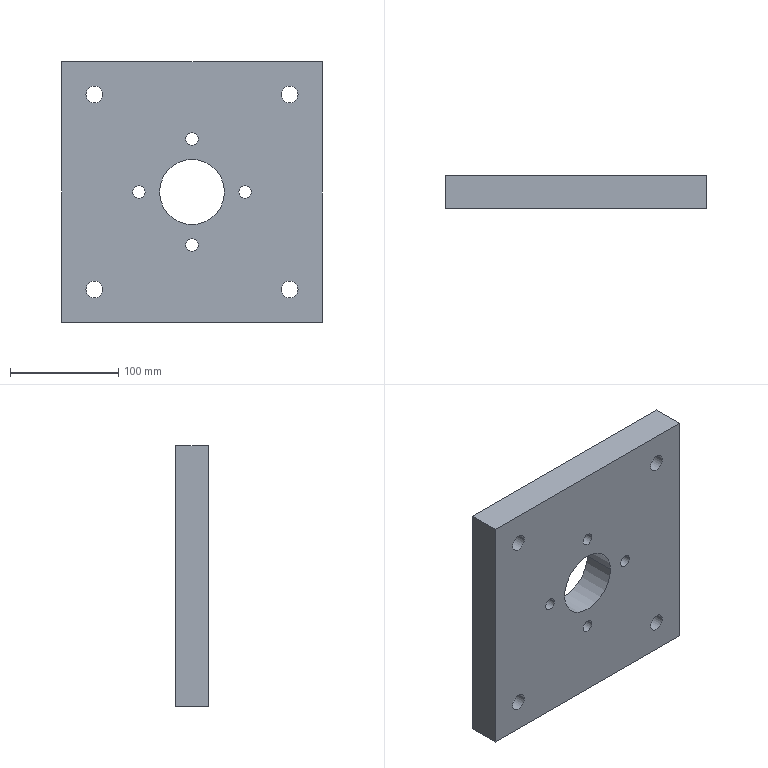Part | STEP file | Scale factor 1[5] | 1 solid | 32 faces | box 240 x 30 x 240 mm | volume 1602106 mm3 | cylinder 22 | plane 6 | cone 4 | commonest cylinder face diameters 11.4 x8 15.6 x8 10.2 x4 60 x2
STEP:
#1=CARTESIAN_POINT('',(-808.738,-386.273,3156.564));
#2=VERTEX_POINT('',#1);
#3=CARTESIAN_POINT('',(-808.738,-381.173,3153.5));
#4=VERTEX_POINT('',#3);
#5=CARTESIAN_POINT('',(-808.738,-381.173,3153.5));
#6=DIRECTION('',(0.,0.8572,-0.515));
#7=VECTOR('',#6,1000.);
#8=LINE('',#5,#7);
#9=EDGE_CURVE('',#2,#4,#8,.T.);
#10=ORIENTED_EDGE('',*,*,#9,.F.);
#11=CARTESIAN_POINT('',(-808.738,-391.373,3153.5));
#12=VERTEX_POINT('',#11);
#13=CARTESIAN_POINT('',(-808.738,-391.373,3153.5));
#14=DIRECTION('',(0.,-0.8572,-0.515));
#15=VECTOR('',#14,1000.);
#16=LINE('',#13,#15);
#17=EDGE_CURVE('',#2,#12,#16,.T.);
#18=ORIENTED_EDGE('',*,*,#17,.T.);
#19=CARTESIAN_POINT('',(-808.738,-386.273,3153.5));
#20=DIRECTION('',(0.,0.,-1.));
#21=DIRECTION('',(0.,1.,0.));
#22=AXIS2_PLACEMENT_3D('',#19,#20,#21);
#23=CIRCLE('',#22,5.1);
#24=EDGE_CURVE('',#12,#4,#23,.T.);
#25=ORIENTED_EDGE('',*,*,#24,.T.);
#26=EDGE_LOOP('',(#10,#18,#25));
#27=FACE_OUTER_BOUND('',#26,.T.);
#28=CARTESIAN_POINT('',(-808.738,-386.273,3153.5));
#29=DIRECTION('',(0.,0.,-1.));
#30=DIRECTION('',(0.,-1.,0.));
#31=AXIS2_PLACEMENT_3D('',#28,#29,#30);
#32=CONICAL_SURFACE('',#31,5.1,1.03);
#33=ADVANCED_FACE('',(#27),#32,.F.);
#34=ORIENTED_EDGE('',*,*,#24,.F.);
#35=CARTESIAN_POINT('',(-808.738,-391.373,3118.5));
#36=VERTEX_POINT('',#35);
#37=CARTESIAN_POINT('',(-808.738,-391.373,3083.5));
#38=DIRECTION('',(0.,0.,-1.));
#39=VECTOR('',#38,1000.);
#40=LINE('',#37,#39);
#41=EDGE_CURVE('',#12,#36,#40,.T.);
#42=ORIENTED_EDGE('',*,*,#41,.T.);
#43=CARTESIAN_POINT('',(-808.738,-381.173,3118.5));
#44=VERTEX_POINT('',#43);
#45=CARTESIAN_POINT('',(-808.738,-386.273,3118.5));
#46=DIRECTION('',(-0.000000001,0.,1.));
#47=DIRECTION('',(0.,-1.,0.));
#48=AXIS2_PLACEMENT_3D('',#45,#46,#47);
#49=CIRCLE('',#48,5.1);
#50=EDGE_CURVE('',#44,#36,#49,.T.);
#51=ORIENTED_EDGE('',*,*,#50,.F.);
#52=CARTESIAN_POINT('',(-808.738,-381.173,3083.5));
#53=DIRECTION('',(0.,0.,-1.));
#54=VECTOR('',#53,1000.);
#55=LINE('',#52,#54);
#56=EDGE_CURVE('',#4,#44,#55,.T.);
#57=ORIENTED_EDGE('',*,*,#56,.F.);
#58=EDGE_LOOP('',(#34,#42,#51,#57));
#59=FACE_OUTER_BOUND('',#58,.T.);
#60=CARTESIAN_POINT('',(-808.738,-386.273,3083.5));
#61=DIRECTION('',(0.,0.,-1.));
#62=DIRECTION('',(0.,-1.,0.));
#63=AXIS2_PLACEMENT_3D('',#60,#61,#62);
#64=CYLINDRICAL_SURFACE('',#63,5.1);
#65=ADVANCED_FACE('',(#59),#64,.F.);
#66=CARTESIAN_POINT('',(-688.738,-386.273,3156.564));
#67=VERTEX_POINT('',#66);
#68=CARTESIAN_POINT('',(-688.738,-381.173,3153.5));
#69=VERTEX_POINT('',#68);
#70=CARTESIAN_POINT('',(-688.738,-381.173,3153.5));
#71=DIRECTION('',(0.,0.8572,-0.515));
#72=VECTOR('',#71,1000.);
#73=LINE('',#70,#72);
#74=EDGE_CURVE('',#67,#69,#73,.T.);
#75=ORIENTED_EDGE('',*,*,#74,.F.);
#76=CARTESIAN_POINT('',(-688.738,-391.373,3153.5));
#77=VERTEX_POINT('',#76);
#78=CARTESIAN_POINT('',(-688.738,-391.373,3153.5));
#79=DIRECTION('',(0.,-0.8572,-0.515));
#80=VECTOR('',#79,1000.);
#81=LINE('',#78,#80);
#82=EDGE_CURVE('',#67,#77,#81,.T.);
#83=ORIENTED_EDGE('',*,*,#82,.T.);
#84=CARTESIAN_POINT('',(-688.738,-386.273,3153.5));
#85=DIRECTION('',(0.,0.,-1.));
#86=DIRECTION('',(0.,1.,0.));
#87=AXIS2_PLACEMENT_3D('',#84,#85,#86);
#88=CIRCLE('',#87,5.1);
#89=EDGE_CURVE('',#77,#69,#88,.T.);
#90=ORIENTED_EDGE('',*,*,#89,.T.);
#91=EDGE_LOOP('',(#75,#83,#90));
#92=FACE_OUTER_BOUND('',#91,.T.);
#93=CARTESIAN_POINT('',(-688.738,-386.273,3153.5));
#94=DIRECTION('',(0.,0.,-1.));
#95=DIRECTION('',(0.,-1.,0.));
#96=AXIS2_PLACEMENT_3D('',#93,#94,#95);
#97=CONICAL_SURFACE('',#96,5.1,1.03);
#98=ADVANCED_FACE('',(#92),#97,.F.);
#99=ORIENTED_EDGE('',*,*,#89,.F.);
#100=CARTESIAN_POINT('',(-688.738,-391.373,3118.5));
#101=VERTEX_POINT('',#100);
#102=CARTESIAN_POINT('',(-688.738,-391.373,3083.5));
#103=DIRECTION('',(0.,0.,-1.));
#104=VECTOR('',#103,1000.);
#105=LINE('',#102,#104);
#106=EDGE_CURVE('',#77,#101,#105,.T.);
#107=ORIENTED_EDGE('',*,*,#106,.T.);
#108=CARTESIAN_POINT('',(-688.738,-381.173,3118.5));
#109=VERTEX_POINT('',#108);
#110=CARTESIAN_POINT('',(-688.738,-386.273,3118.5));
#111=DIRECTION('',(-0.000000001,0.,1.));
#112=DIRECTION('',(0.,-1.,0.));
#113=AXIS2_PLACEMENT_3D('',#110,#111,#112);
#114=CIRCLE('',#113,5.1);
#115=EDGE_CURVE('',#109,#101,#114,.T.);
#116=ORIENTED_EDGE('',*,*,#115,.F.);
#117=CARTESIAN_POINT('',(-688.738,-381.173,3083.5));
#118=DIRECTION('',(0.,0.,-1.));
#119=VECTOR('',#118,1000.);
#120=LINE('',#117,#119);
#121=EDGE_CURVE('',#69,#109,#120,.T.);
#122=ORIENTED_EDGE('',*,*,#121,.F.);
#123=EDGE_LOOP('',(#99,#107,#116,#122));
#124=FACE_OUTER_BOUND('',#123,.T.);
#125=CARTESIAN_POINT('',(-688.738,-386.273,3083.5));
#126=DIRECTION('',(0.,0.,-1.));
#127=DIRECTION('',(0.,-1.,0.));
#128=AXIS2_PLACEMENT_3D('',#125,#126,#127);
#129=CYLINDRICAL_SURFACE('',#128,5.1);
#130=ADVANCED_FACE('',(#124),#129,.F.);
#131=CARTESIAN_POINT('',(-778.738,-401.273,3238.5));
#132=VERTEX_POINT('',#131);
#133=CARTESIAN_POINT('',(-718.738,-401.273,3238.5));
#134=VERTEX_POINT('',#133);
#135=CARTESIAN_POINT('',(-748.738,-401.273,3238.5));
#136=DIRECTION('',(0.,1.,0.));
#137=DIRECTION('',(1.,0.,0.000000001));
#138=AXIS2_PLACEMENT_3D('',#135,#136,#137);
#139=CIRCLE('',#138,30.);
#140=EDGE_CURVE('',#132,#134,#139,.T.);
#141=ORIENTED_EDGE('',*,*,#140,.F.);
#142=CARTESIAN_POINT('',(-778.738,-371.273,3238.5));
#143=VERTEX_POINT('',#142);
#144=CARTESIAN_POINT('',(-778.738,-401.273,3238.5));
#145=DIRECTION('',(0.,1.,0.));
#146=VECTOR('',#145,1000.);
#147=LINE('',#144,#146);
#148=EDGE_CURVE('',#132,#143,#147,.T.);
#149=ORIENTED_EDGE('',*,*,#148,.T.);
#150=CARTESIAN_POINT('',(-718.738,-371.273,3238.5));
#151=VERTEX_POINT('',#150);
#152=CARTESIAN_POINT('',(-748.738,-371.273,3238.5));
#153=DIRECTION('',(0.,1.,0.));
#154=DIRECTION('',(1.,0.,0.000000001));
#155=AXIS2_PLACEMENT_3D('',#152,#153,#154);
#156=CIRCLE('',#155,30.);
#157=EDGE_CURVE('',#143,#151,#156,.T.);
#158=ORIENTED_EDGE('',*,*,#157,.T.);
#159=CARTESIAN_POINT('',(-718.738,-401.273,3238.5));
#160=DIRECTION('',(0.,1.,0.));
#161=VECTOR('',#160,1000.);
#162=LINE('',#159,#161);
#163=EDGE_CURVE('',#134,#151,#162,.T.);
#164=ORIENTED_EDGE('',*,*,#163,.F.);
#165=EDGE_LOOP('',(#141,#149,#158,#164));
#166=FACE_OUTER_BOUND('',#165,.T.);
#167=CARTESIAN_POINT('',(-748.738,-401.273,3238.5));
#168=DIRECTION('',(0.,1.,0.));
#169=DIRECTION('',(-1.,0.,-0.000000001));
#170=AXIS2_PLACEMENT_3D('',#167,#168,#169);
#171=CYLINDRICAL_SURFACE('',#170,30.);
#172=ADVANCED_FACE('',(#166),#171,.F.);
#173=CARTESIAN_POINT('',(-705.538,-401.273,3238.5));
#174=VERTEX_POINT('',#173);
#175=CARTESIAN_POINT('',(-694.138,-401.273,3238.5));
#176=VERTEX_POINT('',#175);
#177=CARTESIAN_POINT('',(-699.838,-401.273,3238.5));
#178=DIRECTION('',(0.,1.,0.));
#179=DIRECTION('',(1.,0.,0.000000001));
#180=AXIS2_PLACEMENT_3D('',#177,#178,#179);
#181=CIRCLE('',#180,5.7);
#182=EDGE_CURVE('',#174,#176,#181,.T.);
#183=ORIENTED_EDGE('',*,*,#182,.F.);
#184=CARTESIAN_POINT('',(-705.538,-371.273,3238.5));
#185=VERTEX_POINT('',#184);
#186=CARTESIAN_POINT('',(-705.538,-401.273,3238.5));
#187=DIRECTION('',(0.,1.,0.));
#188=VECTOR('',#187,1000.);
#189=LINE('',#186,#188);
#190=EDGE_CURVE('',#174,#185,#189,.T.);
#191=ORIENTED_EDGE('',*,*,#190,.T.);
#192=CARTESIAN_POINT('',(-694.138,-371.273,3238.5));
#193=VERTEX_POINT('',#192);
#194=CARTESIAN_POINT('',(-699.838,-371.273,3238.5));
#195=DIRECTION('',(0.,1.,0.));
#196=DIRECTION('',(1.,0.,0.000000001));
#197=AXIS2_PLACEMENT_3D('',#194,#195,#196);
#198=CIRCLE('',#197,5.7);
#199=EDGE_CURVE('',#185,#193,#198,.T.);
#200=ORIENTED_EDGE('',*,*,#199,.T.);
#201=CARTESIAN_POINT('',(-694.138,-401.273,3238.5));
#202=DIRECTION('',(0.,1.,0.));
#203=VECTOR('',#202,1000.);
#204=LINE('',#201,#203);
#205=EDGE_CURVE('',#176,#193,#204,.T.);
#206=ORIENTED_EDGE('',*,*,#205,.F.);
#207=EDGE_LOOP('',(#183,#191,#200,#206));
#208=FACE_OUTER_BOUND('',#207,.T.);
#209=CARTESIAN_POINT('',(-699.838,-401.273,3238.5));
#210=DIRECTION('',(0.,1.,0.));
#211=DIRECTION('',(-1.,0.,-0.000000001));
#212=AXIS2_PLACEMENT_3D('',#209,#210,#211);
#213=CYLINDRICAL_SURFACE('',#212,5.7);
#214=ADVANCED_FACE('',(#208),#213,.F.);
#215=CARTESIAN_POINT('',(-803.338,-401.273,3238.5));
#216=VERTEX_POINT('',#215);
#217=CARTESIAN_POINT('',(-791.938,-401.273,3238.5));
#218=VERTEX_POINT('',#217);
#219=CARTESIAN_POINT('',(-797.638,-401.273,3238.5));
#220=DIRECTION('',(0.,1.,0.));
#221=DIRECTION('',(1.,0.,0.000000001));
#222=AXIS2_PLACEMENT_3D('',#219,#220,#221);
#223=CIRCLE('',#222,5.7);
#224=EDGE_CURVE('',#216,#218,#223,.T.);
#225=ORIENTED_EDGE('',*,*,#224,.F.);
#226=CARTESIAN_POINT('',(-803.338,-371.273,3238.5));
#227=VERTEX_POINT('',#226);
#228=CARTESIAN_POINT('',(-803.338,-401.273,3238.5));
#229=DIRECTION('',(0.,1.,0.));
#230=VECTOR('',#229,1000.);
#231=LINE('',#228,#230);
#232=EDGE_CURVE('',#216,#227,#231,.T.);
#233=ORIENTED_EDGE('',*,*,#232,.T.);
#234=CARTESIAN_POINT('',(-791.938,-371.273,3238.5));
#235=VERTEX_POINT('',#234);
#236=CARTESIAN_POINT('',(-797.638,-371.273,3238.5));
#237=DIRECTION('',(0.,1.,0.));
#238=DIRECTION('',(1.,0.,0.000000001));
#239=AXIS2_PLACEMENT_3D('',#236,#237,#238);
#240=CIRCLE('',#239,5.7);
#241=EDGE_CURVE('',#227,#235,#240,.T.);
#242=ORIENTED_EDGE('',*,*,#241,.T.);
#243=CARTESIAN_POINT('',(-791.938,-401.273,3238.5));
#244=DIRECTION('',(0.,1.,0.));
#245=VECTOR('',#244,1000.);
#246=LINE('',#243,#245);
#247=EDGE_CURVE('',#218,#235,#246,.T.);
#248=ORIENTED_EDGE('',*,*,#247,.F.);
#249=EDGE_LOOP('',(#225,#233,#242,#248));
#250=FACE_OUTER_BOUND('',#249,.T.);
#251=CARTESIAN_POINT('',(-797.638,-401.273,3238.5));
#252=DIRECTION('',(0.,1.,0.));
#253=DIRECTION('',(-1.,0.,-0.000000001));
#254=AXIS2_PLACEMENT_3D('',#251,#252,#253);
#255=CYLINDRICAL_SURFACE('',#254,5.7);
#256=ADVANCED_FACE('',(#250),#255,.F.);
#257=CARTESIAN_POINT('',(-754.438,-401.273,3287.4));
#258=VERTEX_POINT('',#257);
#259=CARTESIAN_POINT('',(-743.038,-401.273,3287.4));
#260=VERTEX_POINT('',#259);
#261=CARTESIAN_POINT('',(-748.738,-401.273,3287.4));
#262=DIRECTION('',(0.,1.,0.));
#263=DIRECTION('',(1.,0.,0.000000001));
#264=AXIS2_PLACEMENT_3D('',#261,#262,#263);
#265=CIRCLE('',#264,5.7);
#266=EDGE_CURVE('',#258,#260,#265,.T.);
#267=ORIENTED_EDGE('',*,*,#266,.F.);
#268=CARTESIAN_POINT('',(-754.438,-371.273,3287.4));
#269=VERTEX_POINT('',#268);
#270=CARTESIAN_POINT('',(-754.438,-401.273,3287.4));
#271=DIRECTION('',(0.,1.,0.));
#272=VECTOR('',#271,1000.);
#273=LINE('',#270,#272);
#274=EDGE_CURVE('',#258,#269,#273,.T.);
#275=ORIENTED_EDGE('',*,*,#274,.T.);
#276=CARTESIAN_POINT('',(-743.038,-371.273,3287.4));
#277=VERTEX_POINT('',#276);
#278=CARTESIAN_POINT('',(-748.738,-371.273,3287.4));
#279=DIRECTION('',(0.,1.,0.));
#280=DIRECTION('',(1.,0.,0.000000001));
#281=AXIS2_PLACEMENT_3D('',#278,#279,#280);
#282=CIRCLE('',#281,5.7);
#283=EDGE_CURVE('',#269,#277,#282,.T.);
#284=ORIENTED_EDGE('',*,*,#283,.T.);
#285=CARTESIAN_POINT('',(-743.038,-401.273,3287.4));
#286=DIRECTION('',(0.,1.,0.));
#287=VECTOR('',#286,1000.);
#288=LINE('',#285,#287);
#289=EDGE_CURVE('',#260,#277,#288,.T.);
#290=ORIENTED_EDGE('',*,*,#289,.F.);
#291=EDGE_LOOP('',(#267,#275,#284,#290));
#292=FACE_OUTER_BOUND('',#291,.T.);
#293=CARTESIAN_POINT('',(-748.738,-401.273,3287.4));
#294=DIRECTION('',(0.,1.,0.));
#295=DIRECTION('',(-1.,0.,-0.000000001));
#296=AXIS2_PLACEMENT_3D('',#293,#294,#295);
#297=CYLINDRICAL_SURFACE('',#296,5.7);
#298=ADVANCED_FACE('',(#292),#297,.F.);
#299=CARTESIAN_POINT('',(-754.438,-401.273,3189.6));
#300=VERTEX_POINT('',#299);
#301=CARTESIAN_POINT('',(-743.038,-401.273,3189.6));
#302=VERTEX_POINT('',#301);
#303=CARTESIAN_POINT('',(-748.738,-401.273,3189.6));
#304=DIRECTION('',(0.,1.,0.));
#305=DIRECTION('',(1.,0.,0.000000001));
#306=AXIS2_PLACEMENT_3D('',#303,#304,#305);
#307=CIRCLE('',#306,5.7);
#308=EDGE_CURVE('',#300,#302,#307,.T.);
#309=ORIENTED_EDGE('',*,*,#308,.F.);
#310=CARTESIAN_POINT('',(-754.438,-371.273,3189.6));
#311=VERTEX_POINT('',#310);
#312=CARTESIAN_POINT('',(-754.438,-401.273,3189.6));
#313=DIRECTION('',(0.,1.,0.));
#314=VECTOR('',#313,1000.);
#315=LINE('',#312,#314);
#316=EDGE_CURVE('',#300,#311,#315,.T.);
#317=ORIENTED_EDGE('',*,*,#316,.T.);
#318=CARTESIAN_POINT('',(-743.038,-371.273,3189.6));
#319=VERTEX_POINT('',#318);
#320=CARTESIAN_POINT('',(-748.738,-371.273,3189.6));
#321=DIRECTION('',(0.,1.,0.));
#322=DIRECTION('',(1.,0.,0.000000001));
#323=AXIS2_PLACEMENT_3D('',#320,#321,#322);
#324=CIRCLE('',#323,5.7);
#325=EDGE_CURVE('',#311,#319,#324,.T.);
#326=ORIENTED_EDGE('',*,*,#325,.T.);
#327=CARTESIAN_POINT('',(-743.038,-401.273,3189.6));
#328=DIRECTION('',(0.,1.,0.));
#329=VECTOR('',#328,1000.);
#330=LINE('',#327,#329);
#331=EDGE_CURVE('',#302,#319,#330,.T.);
#332=ORIENTED_EDGE('',*,*,#331,.F.);
#333=EDGE_LOOP('',(#309,#317,#326,#332));
#334=FACE_OUTER_BOUND('',#333,.T.);
#335=CARTESIAN_POINT('',(-748.738,-401.273,3189.6));
#336=DIRECTION('',(0.,1.,0.));
#337=DIRECTION('',(-1.,0.,-0.000000001));
#338=AXIS2_PLACEMENT_3D('',#335,#336,#337);
#339=CYLINDRICAL_SURFACE('',#338,5.7);
#340=ADVANCED_FACE('',(#334),#339,.F.);
#341=CARTESIAN_POINT('',(-846.538,-401.273,3148.5));
#342=VERTEX_POINT('',#341);
#343=CARTESIAN_POINT('',(-830.938,-401.273,3148.5));
#344=VERTEX_POINT('',#343);
#345=CARTESIAN_POINT('',(-838.738,-401.273,3148.5));
#346=DIRECTION('',(0.,1.,0.));
#347=DIRECTION('',(1.,0.,0.000000001));
#348=AXIS2_PLACEMENT_3D('',#345,#346,#347);
#349=CIRCLE('',#348,7.8);
#350=EDGE_CURVE('',#342,#344,#349,.T.);
#351=ORIENTED_EDGE('',*,*,#350,.F.);
#352=CARTESIAN_POINT('',(-846.538,-371.273,3148.5));
#353=VERTEX_POINT('',#352);
#354=CARTESIAN_POINT('',(-846.538,-401.273,3148.5));
#355=DIRECTION('',(0.,1.,0.));
#356=VECTOR('',#355,1000.);
#357=LINE('',#354,#356);
#358=EDGE_CURVE('',#342,#353,#357,.T.);
#359=ORIENTED_EDGE('',*,*,#358,.T.);
#360=CARTESIAN_POINT('',(-830.938,-371.273,3148.5));
#361=VERTEX_POINT('',#360);
#362=CARTESIAN_POINT('',(-838.738,-371.273,3148.5));
#363=DIRECTION('',(0.,1.,0.));
#364=DIRECTION('',(1.,0.,0.000000001));
#365=AXIS2_PLACEMENT_3D('',#362,#363,#364);
#366=CIRCLE('',#365,7.8);
#367=EDGE_CURVE('',#353,#361,#366,.T.);
#368=ORIENTED_EDGE('',*,*,#367,.T.);
#369=CARTESIAN_POINT('',(-830.938,-401.273,3148.5));
#370=DIRECTION('',(0.,1.,0.));
#371=VECTOR('',#370,1000.);
#372=LINE('',#369,#371);
#373=EDGE_CURVE('',#344,#361,#372,.T.);
#374=ORIENTED_EDGE('',*,*,#373,.F.);
#375=EDGE_LOOP('',(#351,#359,#368,#374));
#376=FACE_OUTER_BOUND('',#375,.T.);
#377=CARTESIAN_POINT('',(-838.738,-401.273,3148.5));
#378=DIRECTION('',(0.,1.,0.));
#379=DIRECTION('',(-1.,0.,-0.000000001));
#380=AXIS2_PLACEMENT_3D('',#377,#378,#379);
#381=CYLINDRICAL_SURFACE('',#380,7.8);
#382=ADVANCED_FACE('',(#376),#381,.F.);
#383=CARTESIAN_POINT('',(-846.538,-401.273,3328.5));
#384=VERTEX_POINT('',#383);
#385=CARTESIAN_POINT('',(-830.938,-401.273,3328.5));
#386=VERTEX_POINT('',#385);
#387=CARTESIAN_POINT('',(-838.738,-401.273,3328.5));
#388=DIRECTION('',(0.,1.,0.));
#389=DIRECTION('',(1.,0.,0.000000001));
#390=AXIS2_PLACEMENT_3D('',#387,#388,#389);
#391=CIRCLE('',#390,7.8);
#392=EDGE_CURVE('',#384,#386,#391,.T.);
#393=ORIENTED_EDGE('',*,*,#392,.F.);
#394=CARTESIAN_POINT('',(-846.538,-371.273,3328.5));
#395=VERTEX_POINT('',#394);
#396=CARTESIAN_POINT('',(-846.538,-401.273,3328.5));
#397=DIRECTION('',(0.,1.,0.));
#398=VECTOR('',#397,1000.);
#399=LINE('',#396,#398);
#400=EDGE_CURVE('',#384,#395,#399,.T.);
#401=ORIENTED_EDGE('',*,*,#400,.T.);
#402=CARTESIAN_POINT('',(-830.938,-371.273,3328.5));
#403=VERTEX_POINT('',#402);
#404=CARTESIAN_POINT('',(-838.738,-371.273,3328.5));
#405=DIRECTION('',(0.,1.,0.));
#406=DIRECTION('',(1.,0.,0.000000001));
#407=AXIS2_PLACEMENT_3D('',#404,#405,#406);
#408=CIRCLE('',#407,7.8);
#409=EDGE_CURVE('',#395,#403,#408,.T.);
#410=ORIENTED_EDGE('',*,*,#409,.T.);
#411=CARTESIAN_POINT('',(-830.938,-401.273,3328.5));
#412=DIRECTION('',(0.,1.,0.));
#413=VECTOR('',#412,1000.);
#414=LINE('',#411,#413);
#415=EDGE_CURVE('',#386,#403,#414,.T.);
#416=ORIENTED_EDGE('',*,*,#415,.F.);
#417=EDGE_LOOP('',(#393,#401,#410,#416));
#418=FACE_OUTER_BOUND('',#417,.T.);
#419=CARTESIAN_POINT('',(-838.738,-401.273,3328.5));
#420=DIRECTION('',(0.,1.,0.));
#421=DIRECTION('',(-1.,0.,-0.000000001));
#422=AXIS2_PLACEMENT_3D('',#419,#420,#421);
#423=CYLINDRICAL_SURFACE('',#422,7.8);
#424=ADVANCED_FACE('',(#418),#423,.F.);
#425=CARTESIAN_POINT('',(-666.538,-401.273,3328.5));
#426=VERTEX_POINT('',#425);
#427=CARTESIAN_POINT('',(-650.938,-401.273,3328.5));
#428=VERTEX_POINT('',#427);
#429=CARTESIAN_POINT('',(-658.738,-401.273,3328.5));
#430=DIRECTION('',(0.,1.,0.));
#431=DIRECTION('',(1.,0.,0.000000001));
#432=AXIS2_PLACEMENT_3D('',#429,#430,#431);
#433=CIRCLE('',#432,7.8);
#434=EDGE_CURVE('',#426,#428,#433,.T.);
#435=ORIENTED_EDGE('',*,*,#434,.F.);
#436=CARTESIAN_POINT('',(-666.538,-371.273,3328.5));
#437=VERTEX_POINT('',#436);
#438=CARTESIAN_POINT('',(-666.538,-401.273,3328.5));
#439=DIRECTION('',(0.,1.,0.));
#440=VECTOR('',#439,1000.);
#441=LINE('',#438,#440);
#442=EDGE_CURVE('',#426,#437,#441,.T.);
#443=ORIENTED_EDGE('',*,*,#442,.T.);
#444=CARTESIAN_POINT('',(-650.938,-371.273,3328.5));
#445=VERTEX_POINT('',#444);
#446=CARTESIAN_POINT('',(-658.738,-371.273,3328.5));
#447=DIRECTION('',(0.,1.,0.));
#448=DIRECTION('',(1.,0.,0.000000001));
#449=AXIS2_PLACEMENT_3D('',#446,#447,#448);
#450=CIRCLE('',#449,7.8);
#451=EDGE_CURVE('',#437,#445,#450,.T.);
#452=ORIENTED_EDGE('',*,*,#451,.T.);
#453=CARTESIAN_POINT('',(-650.938,-401.273,3328.5));
#454=DIRECTION('',(0.,1.,0.));
#455=VECTOR('',#454,1000.);
#456=LINE('',#453,#455);
#457=EDGE_CURVE('',#428,#445,#456,.T.);
#458=ORIENTED_EDGE('',*,*,#457,.F.);
#459=EDGE_LOOP('',(#435,#443,#452,#458));
#460=FACE_OUTER_BOUND('',#459,.T.);
#461=CARTESIAN_POINT('',(-658.738,-401.273,3328.5));
#462=DIRECTION('',(0.,1.,0.));
#463=DIRECTION('',(-1.,0.,-0.000000001));
#464=AXIS2_PLACEMENT_3D('',#461,#462,#463);
#465=CYLINDRICAL_SURFACE('',#464,7.8);
#466=ADVANCED_FACE('',(#460),#465,.F.);
#467=CARTESIAN_POINT('',(-666.538,-401.273,3148.5));
#468=VERTEX_POINT('',#467);
#469=CARTESIAN_POINT('',(-650.938,-401.273,3148.5));
#470=VERTEX_POINT('',#469);
#471=CARTESIAN_POINT('',(-658.738,-401.273,3148.5));
#472=DIRECTION('',(0.,1.,0.));
#473=DIRECTION('',(1.,0.,0.000000001));
#474=AXIS2_PLACEMENT_3D('',#471,#472,#473);
#475=CIRCLE('',#474,7.8);
#476=EDGE_CURVE('',#468,#470,#475,.T.);
#477=ORIENTED_EDGE('',*,*,#476,.F.);
#478=CARTESIAN_POINT('',(-666.538,-371.273,3148.5));
#479=VERTEX_POINT('',#478);
#480=CARTESIAN_POINT('',(-666.538,-401.273,3148.5));
#481=DIRECTION('',(0.,1.,0.));
#482=VECTOR('',#481,1000.);
#483=LINE('',#480,#482);
#484=EDGE_CURVE('',#468,#479,#483,.T.);
#485=ORIENTED_EDGE('',*,*,#484,.T.);
#486=CARTESIAN_POINT('',(-650.938,-371.273,3148.5));
#487=VERTEX_POINT('',#486);
#488=CARTESIAN_POINT('',(-658.738,-371.273,3148.5));
#489=DIRECTION('',(0.,1.,0.));
#490=DIRECTION('',(1.,0.,0.000000001));
#491=AXIS2_PLACEMENT_3D('',#488,#489,#490);
#492=CIRCLE('',#491,7.8);
#493=EDGE_CURVE('',#479,#487,#492,.T.);
#494=ORIENTED_EDGE('',*,*,#493,.T.);
#495=CARTESIAN_POINT('',(-650.938,-401.273,3148.5));
#496=DIRECTION('',(0.,1.,0.));
#497=VECTOR('',#496,1000.);
#498=LINE('',#495,#497);
#499=EDGE_CURVE('',#470,#487,#498,.T.);
#500=ORIENTED_EDGE('',*,*,#499,.F.);
#501=EDGE_LOOP('',(#477,#485,#494,#500));
#502=FACE_OUTER_BOUND('',#501,.T.);
#503=CARTESIAN_POINT('',(-658.738,-401.273,3148.5));
#504=DIRECTION('',(0.,1.,0.));
#505=DIRECTION('',(-1.,0.,-0.000000001));
#506=AXIS2_PLACEMENT_3D('',#503,#504,#505);
#507=CYLINDRICAL_SURFACE('',#506,7.8);
#508=ADVANCED_FACE('',(#502),#507,.F.);
#509=CARTESIAN_POINT('',(-628.738,-401.273,3358.5));
#510=VERTEX_POINT('',#509);
#511=CARTESIAN_POINT('',(-628.738,-401.273,3118.5));
#512=VERTEX_POINT('',#511);
#513=CARTESIAN_POINT('',(-628.738,-401.273,3118.5));
#514=DIRECTION('',(0.000000001,0.,-1.));
#515=VECTOR('',#514,1000.);
#516=LINE('',#513,#515);
#517=EDGE_CURVE('',#510,#512,#516,.T.);
#518=ORIENTED_EDGE('',*,*,#517,.T.);
#519=CARTESIAN_POINT('',(-628.738,-371.273,3118.5));
#520=VERTEX_POINT('',#519);
#521=CARTESIAN_POINT('',(-628.738,-371.273,3118.5));
#522=DIRECTION('',(0.,-1.,0.));
#523=VECTOR('',#522,1000.);
#524=LINE('',#521,#523);
#525=EDGE_CURVE('',#520,#512,#524,.T.);
#526=ORIENTED_EDGE('',*,*,#525,.F.);
#527=CARTESIAN_POINT('',(-628.738,-371.273,3358.5));
#528=VERTEX_POINT('',#527);
#529=CARTESIAN_POINT('',(-628.738,-371.273,3118.5));
#530=DIRECTION('',(0.000000001,0.,-1.));
#531=VECTOR('',#530,1000.);
#532=LINE('',#529,#531);
#533=EDGE_CURVE('',#528,#520,#532,.T.);
#534=ORIENTED_EDGE('',*,*,#533,.F.);
#535=CARTESIAN_POINT('',(-628.738,-371.273,3358.5));
#536=DIRECTION('',(0.,-1.,0.));
#537=VECTOR('',#536,1000.);
#538=LINE('',#535,#537);
#539=EDGE_CURVE('',#528,#510,#538,.T.);
#540=ORIENTED_EDGE('',*,*,#539,.T.);
#541=EDGE_LOOP('',(#518,#526,#534,#540));
#542=FACE_OUTER_BOUND('',#541,.T.);
#543=CARTESIAN_POINT('',(-628.738,-371.273,3118.5));
#544=DIRECTION('',(-1.,0.,-0.000000001));
#545=DIRECTION('',(0.,-1.,0.));
#546=AXIS2_PLACEMENT_3D('',#543,#544,#545);
#547=PLANE('',#546);
#548=ADVANCED_FACE('',(#542),#547,.F.);
#549=ORIENTED_EDGE('',*,*,#50,.T.);
#550=CARTESIAN_POINT('',(-808.738,-386.273,3118.5));
#551=DIRECTION('',(-0.000000001,0.,1.));
#552=DIRECTION('',(0.,-1.,0.));
#553=AXIS2_PLACEMENT_3D('',#550,#551,#552);
#554=CIRCLE('',#553,5.1);
#555=EDGE_CURVE('',#36,#44,#554,.T.);
#556=ORIENTED_EDGE('',*,*,#555,.T.);
#557=EDGE_LOOP('',(#549,#556));
#558=FACE_BOUND('',#557,.T.);
#559=ORIENTED_EDGE('',*,*,#115,.T.);
#560=CARTESIAN_POINT('',(-688.738,-386.273,3118.5));
#561=DIRECTION('',(-0.000000001,0.,1.));
#562=DIRECTION('',(0.,-1.,0.));
#563=AXIS2_PLACEMENT_3D('',#560,#561,#562);
#564=CIRCLE('',#563,5.1);
#565=EDGE_CURVE('',#101,#109,#564,.T.);
#566=ORIENTED_EDGE('',*,*,#565,.T.);
#567=EDGE_LOOP('',(#559,#566));
#568=FACE_BOUND('',#567,.T.);
#569=CARTESIAN_POINT('',(-868.738,-401.273,3118.5));
#570=VERTEX_POINT('',#569);
#571=CARTESIAN_POINT('',(-868.738,-401.273,3118.5));
#572=DIRECTION('',(-1.,0.,-0.000000001));
#573=VECTOR('',#572,1000.);
#574=LINE('',#571,#573);
#575=EDGE_CURVE('',#512,#570,#574,.T.);
#576=ORIENTED_EDGE('',*,*,#575,.T.);
#577=CARTESIAN_POINT('',(-868.738,-371.273,3118.5));
#578=VERTEX_POINT('',#577);
#579=CARTESIAN_POINT('',(-868.738,-371.273,3118.5));
#580=DIRECTION('',(0.,-1.,0.));
#581=VECTOR('',#580,1000.);
#582=LINE('',#579,#581);
#583=EDGE_CURVE('',#578,#570,#582,.T.);
#584=ORIENTED_EDGE('',*,*,#583,.F.);
#585=CARTESIAN_POINT('',(-868.738,-371.273,3118.5));
#586=DIRECTION('',(-1.,0.,-0.000000001));
#587=VECTOR('',#586,1000.);
#588=LINE('',#585,#587);
#589=EDGE_CURVE('',#520,#578,#588,.T.);
#590=ORIENTED_EDGE('',*,*,#589,.F.);
#591=ORIENTED_EDGE('',*,*,#525,.T.);
#592=EDGE_LOOP('',(#576,#584,#590,#591));
#593=FACE_OUTER_BOUND('',#592,.T.);
#594=CARTESIAN_POINT('',(-868.738,-371.273,3118.5));
#595=DIRECTION('',(-0.000000001,0.,1.));
#596=DIRECTION('',(0.,1.,0.));
#597=AXIS2_PLACEMENT_3D('',#594,#595,#596);
#598=PLANE('',#597);
#599=ADVANCED_FACE('',(#558,#568,#593),#598,.F.);
#600=CARTESIAN_POINT('',(-868.738,-401.273,3358.5));
#601=VERTEX_POINT('',#600);
#602=CARTESIAN_POINT('',(-868.738,-401.273,3118.5));
#603=DIRECTION('',(-0.000000001,0.,1.));
#604=VECTOR('',#603,1000.);
#605=LINE('',#602,#604);
#606=EDGE_CURVE('',#570,#601,#605,.T.);
#607=ORIENTED_EDGE('',*,*,#606,.T.);
#608=CARTESIAN_POINT('',(-868.738,-371.273,3358.5));
#609=VERTEX_POINT('',#608);
#610=CARTESIAN_POINT('',(-868.738,-371.273,3358.5));
#611=DIRECTION('',(0.,-1.,0.));
#612=VECTOR('',#611,1000.);
#613=LINE('',#610,#612);
#614=EDGE_CURVE('',#609,#601,#613,.T.);
#615=ORIENTED_EDGE('',*,*,#614,.F.);
#616=CARTESIAN_POINT('',(-868.738,-371.273,3118.5));
#617=DIRECTION('',(-0.000000001,0.,1.));
#618=VECTOR('',#617,1000.);
#619=LINE('',#616,#618);
#620=EDGE_CURVE('',#578,#609,#619,.T.);
#621=ORIENTED_EDGE('',*,*,#620,.F.);
#622=ORIENTED_EDGE('',*,*,#583,.T.);
#623=EDGE_LOOP('',(#607,#615,#621,#622));
#624=FACE_OUTER_BOUND('',#623,.T.);
#625=CARTESIAN_POINT('',(-868.738,-371.273,3118.5));
#626=DIRECTION('',(1.,0.,0.000000001));
#627=DIRECTION('',(-0.000000001,0.,1.));
#628=AXIS2_PLACEMENT_3D('',#625,#626,#627);
#629=PLANE('',#628);
#630=ADVANCED_FACE('',(#624),#629,.F.);
#631=CARTESIAN_POINT('',(-868.738,-401.273,3358.5));
#632=DIRECTION('',(1.,0.,0.000000001));
#633=VECTOR('',#632,1000.);
#634=LINE('',#631,#633);
#635=EDGE_CURVE('',#601,#510,#634,.T.);
#636=ORIENTED_EDGE('',*,*,#635,.T.);
#637=ORIENTED_EDGE('',*,*,#539,.F.);
#638=CARTESIAN_POINT('',(-868.738,-371.273,3358.5));
#639=DIRECTION('',(1.,0.,0.000000001));
#640=VECTOR('',#639,1000.);
#641=LINE('',#638,#640);
#642=EDGE_CURVE('',#609,#528,#641,.T.);
#643=ORIENTED_EDGE('',*,*,#642,.F.);
#644=ORIENTED_EDGE('',*,*,#614,.T.);
#645=EDGE_LOOP('',(#636,#637,#643,#644));
#646=FACE_OUTER_BOUND('',#645,.T.);
#647=CARTESIAN_POINT('',(-868.738,-371.273,3358.5));
#648=DIRECTION('',(0.000000001,0.,-1.));
#649=DIRECTION('',(0.,-1.,0.));
#650=AXIS2_PLACEMENT_3D('',#647,#648,#649);
#651=PLANE('',#650);
#652=ADVANCED_FACE('',(#646),#651,.F.);
#653=CARTESIAN_POINT('',(-748.738,-371.273,3238.5));
#654=DIRECTION('',(0.,1.,0.));
#655=DIRECTION('',(1.,0.,0.000000001));
#656=AXIS2_PLACEMENT_3D('',#653,#654,#655);
#657=CIRCLE('',#656,30.);
#658=EDGE_CURVE('',#151,#143,#657,.T.);
#659=ORIENTED_EDGE('',*,*,#658,.F.);
#660=ORIENTED_EDGE('',*,*,#157,.F.);
#661=EDGE_LOOP('',(#659,#660));
#662=FACE_BOUND('',#661,.T.);
#663=CARTESIAN_POINT('',(-699.838,-371.273,3238.5));
#664=DIRECTION('',(0.,1.,0.));
#665=DIRECTION('',(1.,0.,0.000000001));
#666=AXIS2_PLACEMENT_3D('',#663,#664,#665);
#667=CIRCLE('',#666,5.7);
#668=EDGE_CURVE('',#193,#185,#667,.T.);
#669=ORIENTED_EDGE('',*,*,#668,.F.);
#670=ORIENTED_EDGE('',*,*,#199,.F.);
#671=EDGE_LOOP('',(#669,#670));
#672=FACE_BOUND('',#671,.T.);
#673=CARTESIAN_POINT('',(-797.638,-371.273,3238.5));
#674=DIRECTION('',(0.,1.,0.));
#675=DIRECTION('',(1.,0.,0.000000001));
#676=AXIS2_PLACEMENT_3D('',#673,#674,#675);
#677=CIRCLE('',#676,5.7);
#678=EDGE_CURVE('',#235,#227,#677,.T.);
#679=ORIENTED_EDGE('',*,*,#678,.F.);
#680=ORIENTED_EDGE('',*,*,#241,.F.);
#681=EDGE_LOOP('',(#679,#680));
#682=FACE_BOUND('',#681,.T.);
#683=CARTESIAN_POINT('',(-748.738,-371.273,3287.4));
#684=DIRECTION('',(0.,1.,0.));
#685=DIRECTION('',(1.,0.,0.000000001));
#686=AXIS2_PLACEMENT_3D('',#683,#684,#685);
#687=CIRCLE('',#686,5.7);
#688=EDGE_CURVE('',#277,#269,#687,.T.);
#689=ORIENTED_EDGE('',*,*,#688,.F.);
#690=ORIENTED_EDGE('',*,*,#283,.F.);
#691=EDGE_LOOP('',(#689,#690));
#692=FACE_BOUND('',#691,.T.);
#693=CARTESIAN_POINT('',(-748.738,-371.273,3189.6));
#694=DIRECTION('',(0.,1.,0.));
#695=DIRECTION('',(1.,0.,0.000000001));
#696=AXIS2_PLACEMENT_3D('',#693,#694,#695);
#697=CIRCLE('',#696,5.7);
#698=EDGE_CURVE('',#319,#311,#697,.T.);
#699=ORIENTED_EDGE('',*,*,#698,.F.);
#700=ORIENTED_EDGE('',*,*,#325,.F.);
#701=EDGE_LOOP('',(#699,#700));
#702=FACE_BOUND('',#701,.T.);
#703=CARTESIAN_POINT('',(-838.738,-371.273,3148.5));
#704=DIRECTION('',(0.,1.,0.));
#705=DIRECTION('',(1.,0.,0.000000001));
#706=AXIS2_PLACEMENT_3D('',#703,#704,#705);
#707=CIRCLE('',#706,7.8);
#708=EDGE_CURVE('',#361,#353,#707,.T.);
#709=ORIENTED_EDGE('',*,*,#708,.F.);
#710=ORIENTED_EDGE('',*,*,#367,.F.);
#711=EDGE_LOOP('',(#709,#710));
#712=FACE_BOUND('',#711,.T.);
#713=CARTESIAN_POINT('',(-838.738,-371.273,3328.5));
#714=DIRECTION('',(0.,1.,0.));
#715=DIRECTION('',(1.,0.,0.000000001));
#716=AXIS2_PLACEMENT_3D('',#713,#714,#715);
#717=CIRCLE('',#716,7.8);
#718=EDGE_CURVE('',#403,#395,#717,.T.);
#719=ORIENTED_EDGE('',*,*,#718,.F.);
#720=ORIENTED_EDGE('',*,*,#409,.F.);
#721=EDGE_LOOP('',(#719,#720));
#722=FACE_BOUND('',#721,.T.);
#723=CARTESIAN_POINT('',(-658.738,-371.273,3328.5));
#724=DIRECTION('',(0.,1.,0.));
#725=DIRECTION('',(1.,0.,0.000000001));
#726=AXIS2_PLACEMENT_3D('',#723,#724,#725);
#727=CIRCLE('',#726,7.8);
#728=EDGE_CURVE('',#445,#437,#727,.T.);
#729=ORIENTED_EDGE('',*,*,#728,.F.);
#730=ORIENTED_EDGE('',*,*,#451,.F.);
#731=EDGE_LOOP('',(#729,#730));
#732=FACE_BOUND('',#731,.T.);
#733=CARTESIAN_POINT('',(-658.738,-371.273,3148.5));
#734=DIRECTION('',(0.,1.,0.));
#735=DIRECTION('',(1.,0.,0.000000001));
#736=AXIS2_PLACEMENT_3D('',#733,#734,#735);
#737=CIRCLE('',#736,7.8);
#738=EDGE_CURVE('',#487,#479,#737,.T.);
#739=ORIENTED_EDGE('',*,*,#738,.F.);
#740=ORIENTED_EDGE('',*,*,#493,.F.);
#741=EDGE_LOOP('',(#739,#740));
#742=FACE_BOUND('',#741,.T.);
#743=ORIENTED_EDGE('',*,*,#533,.T.);
#744=ORIENTED_EDGE('',*,*,#589,.T.);
#745=ORIENTED_EDGE('',*,*,#620,.T.);
#746=ORIENTED_EDGE('',*,*,#642,.T.);
#747=EDGE_LOOP('',(#743,#744,#745,#746));
#748=FACE_OUTER_BOUND('',#747,.T.);
#749=CARTESIAN_POINT('',(-748.738,-371.273,3238.5));
#750=DIRECTION('',(0.,1.,0.));
#751=DIRECTION('',(-1.,0.,-0.000000001));
#752=AXIS2_PLACEMENT_3D('',#749,#750,#751);
#753=PLANE('',#752);
#754=ADVANCED_FACE('',(#662,#672,#682,#692,#702,#712,#722,#732,#742,#748),#753,.T.);
#755=CARTESIAN_POINT('',(-748.738,-401.273,3238.5));
#756=DIRECTION('',(0.,1.,0.));
#757=DIRECTION('',(1.,0.,0.000000001));
#758=AXIS2_PLACEMENT_3D('',#755,#756,#757);
#759=CIRCLE('',#758,30.);
#760=EDGE_CURVE('',#134,#132,#759,.T.);
#761=ORIENTED_EDGE('',*,*,#760,.T.);
#762=ORIENTED_EDGE('',*,*,#140,.T.);
#763=EDGE_LOOP('',(#761,#762));
#764=FACE_BOUND('',#763,.T.);
#765=CARTESIAN_POINT('',(-699.838,-401.273,3238.5));
#766=DIRECTION('',(0.,1.,0.));
#767=DIRECTION('',(1.,0.,0.000000001));
#768=AXIS2_PLACEMENT_3D('',#765,#766,#767);
#769=CIRCLE('',#768,5.7);
#770=EDGE_CURVE('',#176,#174,#769,.T.);
#771=ORIENTED_EDGE('',*,*,#770,.T.);
#772=ORIENTED_EDGE('',*,*,#182,.T.);
#773=EDGE_LOOP('',(#771,#772));
#774=FACE_BOUND('',#773,.T.);
#775=CARTESIAN_POINT('',(-797.638,-401.273,3238.5));
#776=DIRECTION('',(0.,1.,0.));
#777=DIRECTION('',(1.,0.,0.000000001));
#778=AXIS2_PLACEMENT_3D('',#775,#776,#777);
#779=CIRCLE('',#778,5.7);
#780=EDGE_CURVE('',#218,#216,#779,.T.);
#781=ORIENTED_EDGE('',*,*,#780,.T.);
#782=ORIENTED_EDGE('',*,*,#224,.T.);
#783=EDGE_LOOP('',(#781,#782));
#784=FACE_BOUND('',#783,.T.);
#785=CARTESIAN_POINT('',(-748.738,-401.273,3287.4));
#786=DIRECTION('',(0.,1.,0.));
#787=DIRECTION('',(1.,0.,0.000000001));
#788=AXIS2_PLACEMENT_3D('',#785,#786,#787);
#789=CIRCLE('',#788,5.7);
#790=EDGE_CURVE('',#260,#258,#789,.T.);
#791=ORIENTED_EDGE('',*,*,#790,.T.);
#792=ORIENTED_EDGE('',*,*,#266,.T.);
#793=EDGE_LOOP('',(#791,#792));
#794=FACE_BOUND('',#793,.T.);
#795=CARTESIAN_POINT('',(-748.738,-401.273,3189.6));
#796=DIRECTION('',(0.,1.,0.));
#797=DIRECTION('',(1.,0.,0.000000001));
#798=AXIS2_PLACEMENT_3D('',#795,#796,#797);
#799=CIRCLE('',#798,5.7);
#800=EDGE_CURVE('',#302,#300,#799,.T.);
#801=ORIENTED_EDGE('',*,*,#800,.T.);
#802=ORIENTED_EDGE('',*,*,#308,.T.);
#803=EDGE_LOOP('',(#801,#802));
#804=FACE_BOUND('',#803,.T.);
#805=CARTESIAN_POINT('',(-838.738,-401.273,3148.5));
#806=DIRECTION('',(0.,1.,0.));
#807=DIRECTION('',(1.,0.,0.000000001));
#808=AXIS2_PLACEMENT_3D('',#805,#806,#807);
#809=CIRCLE('',#808,7.8);
#810=EDGE_CURVE('',#344,#342,#809,.T.);
#811=ORIENTED_EDGE('',*,*,#810,.T.);
#812=ORIENTED_EDGE('',*,*,#350,.T.);
#813=EDGE_LOOP('',(#811,#812));
#814=FACE_BOUND('',#813,.T.);
#815=CARTESIAN_POINT('',(-838.738,-401.273,3328.5));
#816=DIRECTION('',(0.,1.,0.));
#817=DIRECTION('',(1.,0.,0.000000001));
#818=AXIS2_PLACEMENT_3D('',#815,#816,#817);
#819=CIRCLE('',#818,7.8);
#820=EDGE_CURVE('',#386,#384,#819,.T.);
#821=ORIENTED_EDGE('',*,*,#820,.T.);
#822=ORIENTED_EDGE('',*,*,#392,.T.);
#823=EDGE_LOOP('',(#821,#822));
#824=FACE_BOUND('',#823,.T.);
#825=CARTESIAN_POINT('',(-658.738,-401.273,3328.5));
#826=DIRECTION('',(0.,1.,0.));
#827=DIRECTION('',(1.,0.,0.000000001));
#828=AXIS2_PLACEMENT_3D('',#825,#826,#827);
#829=CIRCLE('',#828,7.8);
#830=EDGE_CURVE('',#428,#426,#829,.T.);
#831=ORIENTED_EDGE('',*,*,#830,.T.);
#832=ORIENTED_EDGE('',*,*,#434,.T.);
#833=EDGE_LOOP('',(#831,#832));
#834=FACE_BOUND('',#833,.T.);
#835=CARTESIAN_POINT('',(-658.738,-401.273,3148.5));
#836=DIRECTION('',(0.,1.,0.));
#837=DIRECTION('',(1.,0.,0.000000001));
#838=AXIS2_PLACEMENT_3D('',#835,#836,#837);
#839=CIRCLE('',#838,7.8);
#840=EDGE_CURVE('',#470,#468,#839,.T.);
#841=ORIENTED_EDGE('',*,*,#840,.T.);
#842=ORIENTED_EDGE('',*,*,#476,.T.);
#843=EDGE_LOOP('',(#841,#842));
#844=FACE_BOUND('',#843,.T.);
#845=ORIENTED_EDGE('',*,*,#517,.F.);
#846=ORIENTED_EDGE('',*,*,#635,.F.);
#847=ORIENTED_EDGE('',*,*,#606,.F.);
#848=ORIENTED_EDGE('',*,*,#575,.F.);
#849=EDGE_LOOP('',(#845,#846,#847,#848));
#850=FACE_OUTER_BOUND('',#849,.T.);
#851=CARTESIAN_POINT('',(-748.738,-401.273,3238.5));
#852=DIRECTION('',(0.,1.,0.));
#853=DIRECTION('',(-1.,0.,-0.000000001));
#854=AXIS2_PLACEMENT_3D('',#851,#852,#853);
#855=PLANE('',#854);
#856=ADVANCED_FACE('',(#764,#774,#784,#794,#804,#814,#824,#834,#844,#850),#855,.F.);
#857=ORIENTED_EDGE('',*,*,#484,.F.);
#858=ORIENTED_EDGE('',*,*,#840,.F.);
#859=ORIENTED_EDGE('',*,*,#499,.T.);
#860=ORIENTED_EDGE('',*,*,#738,.T.);
#861=EDGE_LOOP('',(#857,#858,#859,#860));
#862=FACE_OUTER_BOUND('',#861,.T.);
#863=CARTESIAN_POINT('',(-658.738,-401.273,3148.5));
#864=DIRECTION('',(0.,1.,0.));
#865=DIRECTION('',(-1.,0.,-0.000000001));
#866=AXIS2_PLACEMENT_3D('',#863,#864,#865);
#867=CYLINDRICAL_SURFACE('',#866,7.8);
#868=ADVANCED_FACE('',(#862),#867,.F.);
#869=ORIENTED_EDGE('',*,*,#442,.F.);
#870=ORIENTED_EDGE('',*,*,#830,.F.);
#871=ORIENTED_EDGE('',*,*,#457,.T.);
#872=ORIENTED_EDGE('',*,*,#728,.T.);
#873=EDGE_LOOP('',(#869,#870,#871,#872));
#874=FACE_OUTER_BOUND('',#873,.T.);
#875=CARTESIAN_POINT('',(-658.738,-401.273,3328.5));
#876=DIRECTION('',(0.,1.,0.));
#877=DIRECTION('',(-1.,0.,-0.000000001));
#878=AXIS2_PLACEMENT_3D('',#875,#876,#877);
#879=CYLINDRICAL_SURFACE('',#878,7.8);
#880=ADVANCED_FACE('',(#874),#879,.F.);
#881=ORIENTED_EDGE('',*,*,#400,.F.);
#882=ORIENTED_EDGE('',*,*,#820,.F.);
#883=ORIENTED_EDGE('',*,*,#415,.T.);
#884=ORIENTED_EDGE('',*,*,#718,.T.);
#885=EDGE_LOOP('',(#881,#882,#883,#884));
#886=FACE_OUTER_BOUND('',#885,.T.);
#887=CARTESIAN_POINT('',(-838.738,-401.273,3328.5));
#888=DIRECTION('',(0.,1.,0.));
#889=DIRECTION('',(-1.,0.,-0.000000001));
#890=AXIS2_PLACEMENT_3D('',#887,#888,#889);
#891=CYLINDRICAL_SURFACE('',#890,7.8);
#892=ADVANCED_FACE('',(#886),#891,.F.);
#893=ORIENTED_EDGE('',*,*,#358,.F.);
#894=ORIENTED_EDGE('',*,*,#810,.F.);
#895=ORIENTED_EDGE('',*,*,#373,.T.);
#896=ORIENTED_EDGE('',*,*,#708,.T.);
#897=EDGE_LOOP('',(#893,#894,#895,#896));
#898=FACE_OUTER_BOUND('',#897,.T.);
#899=CARTESIAN_POINT('',(-838.738,-401.273,3148.5));
#900=DIRECTION('',(0.,1.,0.));
#901=DIRECTION('',(-1.,0.,-0.000000001));
#902=AXIS2_PLACEMENT_3D('',#899,#900,#901);
#903=CYLINDRICAL_SURFACE('',#902,7.8);
#904=ADVANCED_FACE('',(#898),#903,.F.);
#905=ORIENTED_EDGE('',*,*,#316,.F.);
#906=ORIENTED_EDGE('',*,*,#800,.F.);
#907=ORIENTED_EDGE('',*,*,#331,.T.);
#908=ORIENTED_EDGE('',*,*,#698,.T.);
#909=EDGE_LOOP('',(#905,#906,#907,#908));
#910=FACE_OUTER_BOUND('',#909,.T.);
#911=CARTESIAN_POINT('',(-748.738,-401.273,3189.6));
#912=DIRECTION('',(0.,1.,0.));
#913=DIRECTION('',(-1.,0.,-0.000000001));
#914=AXIS2_PLACEMENT_3D('',#911,#912,#913);
#915=CYLINDRICAL_SURFACE('',#914,5.7);
#916=ADVANCED_FACE('',(#910),#915,.F.);
#917=ORIENTED_EDGE('',*,*,#274,.F.);
#918=ORIENTED_EDGE('',*,*,#790,.F.);
#919=ORIENTED_EDGE('',*,*,#289,.T.);
#920=ORIENTED_EDGE('',*,*,#688,.T.);
#921=EDGE_LOOP('',(#917,#918,#919,#920));
#922=FACE_OUTER_BOUND('',#921,.T.);
#923=CARTESIAN_POINT('',(-748.738,-401.273,3287.4));
#924=DIRECTION('',(0.,1.,0.));
#925=DIRECTION('',(-1.,0.,-0.000000001));
#926=AXIS2_PLACEMENT_3D('',#923,#924,#925);
#927=CYLINDRICAL_SURFACE('',#926,5.7);
#928=ADVANCED_FACE('',(#922),#927,.F.);
#929=ORIENTED_EDGE('',*,*,#232,.F.);
#930=ORIENTED_EDGE('',*,*,#780,.F.);
#931=ORIENTED_EDGE('',*,*,#247,.T.);
#932=ORIENTED_EDGE('',*,*,#678,.T.);
#933=EDGE_LOOP('',(#929,#930,#931,#932));
#934=FACE_OUTER_BOUND('',#933,.T.);
#935=CARTESIAN_POINT('',(-797.638,-401.273,3238.5));
#936=DIRECTION('',(0.,1.,0.));
#937=DIRECTION('',(-1.,0.,-0.000000001));
#938=AXIS2_PLACEMENT_3D('',#935,#936,#937);
#939=CYLINDRICAL_SURFACE('',#938,5.7);
#940=ADVANCED_FACE('',(#934),#939,.F.);
#941=ORIENTED_EDGE('',*,*,#190,.F.);
#942=ORIENTED_EDGE('',*,*,#770,.F.);
#943=ORIENTED_EDGE('',*,*,#205,.T.);
#944=ORIENTED_EDGE('',*,*,#668,.T.);
#945=EDGE_LOOP('',(#941,#942,#943,#944));
#946=FACE_OUTER_BOUND('',#945,.T.);
#947=CARTESIAN_POINT('',(-699.838,-401.273,3238.5));
#948=DIRECTION('',(0.,1.,0.));
#949=DIRECTION('',(-1.,0.,-0.000000001));
#950=AXIS2_PLACEMENT_3D('',#947,#948,#949);
#951=CYLINDRICAL_SURFACE('',#950,5.7);
#952=ADVANCED_FACE('',(#946),#951,.F.);
#953=ORIENTED_EDGE('',*,*,#148,.F.);
#954=ORIENTED_EDGE('',*,*,#760,.F.);
#955=ORIENTED_EDGE('',*,*,#163,.T.);
#956=ORIENTED_EDGE('',*,*,#658,.T.);
#957=EDGE_LOOP('',(#953,#954,#955,#956));
#958=FACE_OUTER_BOUND('',#957,.T.);
#959=CARTESIAN_POINT('',(-748.738,-401.273,3238.5));
#960=DIRECTION('',(0.,1.,0.));
#961=DIRECTION('',(-1.,0.,-0.000000001));
#962=AXIS2_PLACEMENT_3D('',#959,#960,#961);
#963=CYLINDRICAL_SURFACE('',#962,30.);
#964=ADVANCED_FACE('',(#958),#963,.F.);
#965=ORIENTED_EDGE('',*,*,#106,.F.);
#966=CARTESIAN_POINT('',(-688.738,-386.273,3153.5));
#967=DIRECTION('',(0.,0.,-1.));
#968=DIRECTION('',(0.,1.,0.));
#969=AXIS2_PLACEMENT_3D('',#966,#967,#968);
#970=CIRCLE('',#969,5.1);
#971=EDGE_CURVE('',#69,#77,#970,.T.);
#972=ORIENTED_EDGE('',*,*,#971,.F.);
#973=ORIENTED_EDGE('',*,*,#121,.T.);
#974=ORIENTED_EDGE('',*,*,#565,.F.);
#975=EDGE_LOOP('',(#965,#972,#973,#974));
#976=FACE_OUTER_BOUND('',#975,.T.);
#977=CARTESIAN_POINT('',(-688.738,-386.273,3083.5));
#978=DIRECTION('',(0.,0.,-1.));
#979=DIRECTION('',(0.,-1.,0.));
#980=AXIS2_PLACEMENT_3D('',#977,#978,#979);
#981=CYLINDRICAL_SURFACE('',#980,5.1);
#982=ADVANCED_FACE('',(#976),#981,.F.);
#983=ORIENTED_EDGE('',*,*,#82,.F.);
#984=ORIENTED_EDGE('',*,*,#74,.T.);
#985=ORIENTED_EDGE('',*,*,#971,.T.);
#986=EDGE_LOOP('',(#983,#984,#985));
#987=FACE_OUTER_BOUND('',#986,.T.);
#988=CARTESIAN_POINT('',(-688.738,-386.273,3153.5));
#989=DIRECTION('',(0.,0.,-1.));
#990=DIRECTION('',(0.,-1.,0.));
#991=AXIS2_PLACEMENT_3D('',#988,#989,#990);
#992=CONICAL_SURFACE('',#991,5.1,1.03);
#993=ADVANCED_FACE('',(#987),#992,.F.);
#994=ORIENTED_EDGE('',*,*,#41,.F.);
#995=CARTESIAN_POINT('',(-808.738,-386.273,3153.5));
#996=DIRECTION('',(0.,0.,-1.));
#997=DIRECTION('',(0.,1.,0.));
#998=AXIS2_PLACEMENT_3D('',#995,#996,#997);
#999=CIRCLE('',#998,5.1);
#1000=EDGE_CURVE('',#4,#12,#999,.T.);
#1001=ORIENTED_EDGE('',*,*,#1000,.F.);
#1002=ORIENTED_EDGE('',*,*,#56,.T.);
#1003=ORIENTED_EDGE('',*,*,#555,.F.);
#1004=EDGE_LOOP('',(#994,#1001,#1002,#1003));
#1005=FACE_OUTER_BOUND('',#1004,.T.);
#1006=CARTESIAN_POINT('',(-808.738,-386.273,3083.5));
#1007=DIRECTION('',(0.,0.,-1.));
#1008=DIRECTION('',(0.,-1.,0.));
#1009=AXIS2_PLACEMENT_3D('',#1006,#1007,#1008);
#1010=CYLINDRICAL_SURFACE('',#1009,5.1);
#1011=ADVANCED_FACE('',(#1005),#1010,.F.);
#1012=ORIENTED_EDGE('',*,*,#17,.F.);
#1013=ORIENTED_EDGE('',*,*,#9,.T.);
#1014=ORIENTED_EDGE('',*,*,#1000,.T.);
#1015=EDGE_LOOP('',(#1012,#1013,#1014));
#1016=FACE_OUTER_BOUND('',#1015,.T.);
#1017=CARTESIAN_POINT('',(-808.738,-386.273,3153.5));
#1018=DIRECTION('',(0.,0.,-1.));
#1019=DIRECTION('',(0.,-1.,0.));
#1020=AXIS2_PLACEMENT_3D('',#1017,#1018,#1019);
#1021=CONICAL_SURFACE('',#1020,5.1,1.03);
#1022=ADVANCED_FACE('',(#1016),#1021,.F.);
#1023=CLOSED_SHELL('',(#33,#65,#98,#130,#172,#214,#256,#298,#340,#382,#424,#466,#508,#548,#599,#630,#652,#754,#856,#868,#880,#892,#904,#916,#928,#940,#952,#964,#982,#993,#1011,#1022));
#1024=MANIFOLD_SOLID_BREP('',#1023);
#1025=CARTESIAN_POINT('',(0.,0.,0.));
#1026=DIRECTION('',(0.,0.,1.));
#1027=DIRECTION('',(1.,0.,0.));
#1028=AXIS2_PLACEMENT_3D('',#1025,#1026,#1027);
#1029=(LENGTH_UNIT()NAMED_UNIT(*)SI_UNIT(.MILLI.,.METRE.));
#1030=UNCERTAINTY_MEASURE_WITH_UNIT(LENGTH_MEASURE(0.00001),#1029,'','');
#1031=(NAMED_UNIT(*)PLANE_ANGLE_UNIT()SI_UNIT($,.RADIAN.));
#1032=(NAMED_UNIT(*)SI_UNIT($,.STERADIAN.)SOLID_ANGLE_UNIT());
#1033=(GEOMETRIC_REPRESENTATION_CONTEXT(3)GLOBAL_UNCERTAINTY_ASSIGNED_CONTEXT((#1030))GLOBAL_UNIT_ASSIGNED_CONTEXT((#1029,#1031,#1032))REPRESENTATION_CONTEXT('',''));
#1034=ADVANCED_BREP_SHAPE_REPRESENTATION('',(#1024,#1028),#1033);